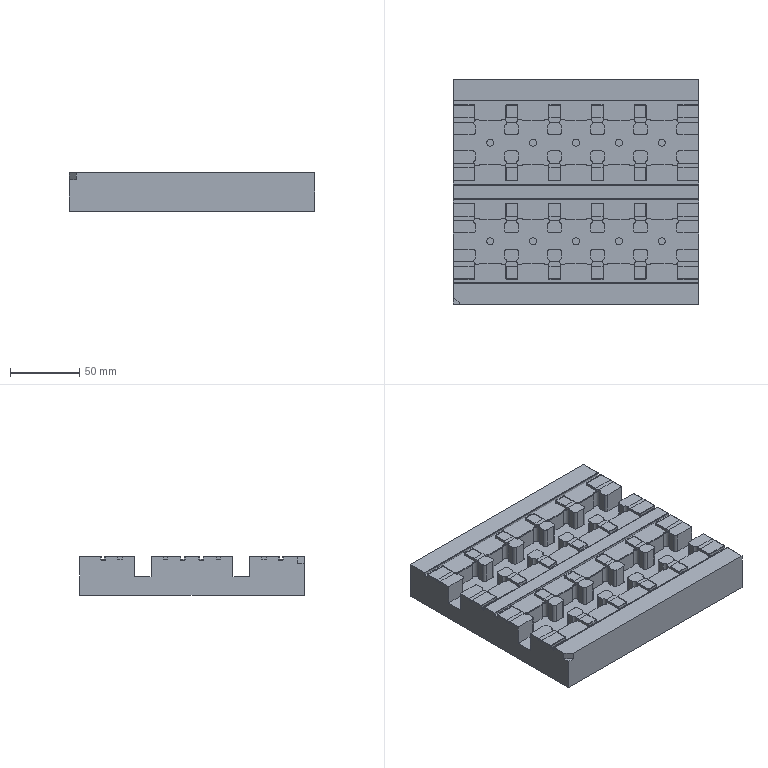NC program | NX | posted by the shop | part box 177 x 162 x 28 mm
Lines 234194 to 237122 of 240480:
N6 T04 M06
(D3  D=3. R=0. H=04 ce=0.05 di=0.02)
(D.N=04 MAX_Z=43. MIN_Z=26.22 Time=39.16M)
T11
G00 G90 G54 X94. Y64.65 M03 S5000
G43 H04 Z43.
M08
Z27.94
G01 X88.5 F1500.
X-88.5
X-94.
G00 Z27.88
G01 X-88.5
X88.5
X94.
G00 Z27.82
G01 X88.5
X-88.5
X-94.
G00 Z27.76
G01 X-88.5
X88.5
X94.
G00 Z27.7
G01 X88.5
X-88.5
X-94.
G00 Z27.64
G01 X-88.5
X88.5
X94.
G00 Z27.58
G01 X88.5
X-88.5
X-94.
G00 Z27.52
G01 X-88.5
X88.5
X94.
G00 Z27.46
G01 X88.5
X-88.5
X-94.
G00 Z27.4
G01 X-88.5
X88.5
X94.
G00 Z27.34
G01 X88.5
X-88.5
X-94.
G00 Z27.28
G01 X-88.5
X88.5
X94.
G00 Z27.22
G01 X88.5
X-88.5
X-94.
G00 Z27.16
G01 X-88.5
X88.5
X94.
G00 Z27.1
G01 X88.5
X-88.5
X-94.
G00 Z27.04
G01 X-88.5
X88.5
X94.
G00 Z26.98
G01 X88.5
X-88.5
X-94.
G00 Z26.92
G01 X-88.5
X88.5
X94.
G00 Z26.86
G01 X88.5
X-88.5
X-94.
G00 Z26.8
G01 X-88.5
X88.5
X94.
G00 Z26.74
G01 X88.5
X-88.5
X-94.
G00 Z26.68
G01 X-88.5
X88.5
X94.
G00 Z26.62
G01 X88.5
X-88.5
X-94.
G00 Z26.56
G01 X-88.5
X88.5
X94.
G00 Z26.5
G01 X88.5
X-88.5
X-94.
G00 Z26.44
G01 X-88.5
X88.5
X94.
G00 Z26.38
G01 X88.5
X-88.5
X-94.
G00 Z26.32
G01 X-88.5
X88.5
X94.
G00 Z26.26
G01 X88.5
X-88.5
X-94.
G00 Z26.22
G01 X-88.5
X88.5
X94.
G00 Z43.
X-94. Y6.55
Z27.94
G01 X-88.5
X88.5
X94.
G00 Z27.88
G01 X88.5
X-88.5
X-94.
G00 Z27.82
G01 X-88.5
X88.5
X94.
G00 Z27.76
G01 X88.5
X-88.5
X-94.
G00 Z27.7
G01 X-88.5
X88.5
X94.
G00 Z27.64
G01 X88.5
X-88.5
X-94.
G00 Z27.58
G01 X-88.5
X88.5
X94.
G00 Z27.52
G01 X88.5
X-88.5
X-94.
G00 Z27.46
G01 X-88.5
X88.5
X94.
G00 Z27.4
G01 X88.5
X-88.5
X-94.
G00 Z27.34
G01 X-88.5
X88.5
X94.
G00 Z27.28
G01 X88.5
X-88.5
X-94.
G00 Z27.22
G01 X-88.5
X88.5
X94.
G00 Z27.16
G01 X88.5
X-88.5
X-94.
G00 Z27.1
G01 X-88.5
X88.5
X94.
G00 Z27.04
G01 X88.5
X-88.5
X-94.
G00 Z26.98
G01 X-88.5
X88.5
X94.
G00 Z26.92
G01 X88.5
X-88.5
X-94.
G00 Z26.86
G01 X-88.5
X88.5
X94.
G00 Z26.8
G01 X88.5
X-88.5
X-94.
G00 Z26.74
G01 X-88.5
X88.5
X94.
G00 Z26.68
G01 X88.5
X-88.5
X-94.
G00 Z26.62
G01 X-88.5
X88.5
X94.
G00 Z26.56
G01 X88.5
X-88.5
X-94.
G00 Z26.5
G01 X-88.5
X88.5
X94.
G00 Z26.44
G01 X88.5
X-88.5
X-94.
G00 Z26.38
G01 X-88.5
X88.5
X94.
G00 Z26.32
G01 X88.5
X-88.5
X-94.
G00 Z26.26
G01 X-88.5
X88.5
X94.
G00 Z26.22
G01 X88.5
X-88.5
X-94.
G00 Z43.
X94. Y-6.55
Z27.94
G01 X88.5
X-88.5
X-94.
G00 Z27.88
G01 X-88.5
X88.5
X94.
G00 Z27.82
G01 X88.5
X-88.5
X-94.
G00 Z27.76
G01 X-88.5
X88.5
X94.
G00 Z27.7
G01 X88.5
X-88.5
X-94.
G00 Z27.64
G01 X-88.5
X88.5
X94.
G00 Z27.58
G01 X88.5
X-88.5
X-94.
G00 Z27.52
G01 X-88.5
X88.5
X94.
G00 Z27.46
G01 X88.5
X-88.5
X-94.
G00 Z27.4
G01 X-88.5
X88.5
X94.
G00 Z27.34
G01 X88.5
X-88.5
X-94.
G00 Z27.28
G01 X-88.5
X88.5
X94.
G00 Z27.22
G01 X88.5
X-88.5
X-94.
G00 Z27.16
G01 X-88.5
X88.5
X94.
G00 Z27.1
G01 X88.5
X-88.5
X-94.
G00 Z27.04
G01 X-88.5
X88.5
X94.
G00 Z26.98
G01 X88.5
X-88.5
X-94.
G00 Z26.92
G01 X-88.5
X88.5
X94.
G00 Z26.86
G01 X88.5
X-88.5
X-94.
G00 Z26.8
G01 X-88.5
X88.5
X94.
G00 Z26.74
G01 X88.5
X-88.5
X-94.
G00 Z26.68
G01 X-88.5
X88.5
X94.
G00 Z26.62
G01 X88.5
X-88.5
X-94.
G00 Z26.56
G01 X-88.5
X88.5
X94.
G00 Z26.5
G01 X88.5
X-88.5
X-94.
G00 Z26.44
G01 X-88.5
X88.5
X94.
G00 Z26.38
G01 X88.5
X-88.5
X-94.
G00 Z26.32
G01 X-88.5
X88.5
X94.
G00 Z26.26
G01 X88.5
X-88.5
X-94.
G00 Z26.22
G01 X-88.5
X88.5
X94.
G00 Z43.
X-94. Y-64.65
Z27.94
G01 X-88.5
X88.5
X94.
G00 Z27.88
G01 X88.5
X-88.5
X-94.
G00 Z27.82
G01 X-88.5
X88.5
X94.
G00 Z27.76
G01 X88.5
X-88.5
X-94.
G00 Z27.7
G01 X-88.5
X88.5
X94.
G00 Z27.64
G01 X88.5
X-88.5
X-94.
G00 Z27.58
G01 X-88.5
X88.5
X94.
G00 Z27.52
G01 X88.5
X-88.5
X-94.
G00 Z27.46
G01 X-88.5
X88.5
X94.
G00 Z27.4
G01 X88.5
X-88.5
X-94.
G00 Z27.34
G01 X-88.5
X88.5
X94.
G00 Z27.28
G01 X88.5
X-88.5
X-94.
G00 Z27.22
G01 X-88.5
X88.5
X94.
G00 Z27.16
G01 X88.5
X-88.5
X-94.
G00 Z27.1
G01 X-88.5
X88.5
X94.
G00 Z27.04
G01 X88.5
X-88.5
X-94.
G00 Z26.98
G01 X-88.5
X88.5
X94.
G00 Z26.92
G01 X88.5
X-88.5
X-94.
G00 Z26.86
G01 X-88.5
X88.5
X94.
G00 Z26.8
G01 X88.5
X-88.5
X-94.
G00 Z26.74
G01 X-88.5
X88.5
X94.
G00 Z26.68
G01 X88.5
X-88.5
X-94.
G00 Z26.62
G01 X-88.5
X88.5
X94.
G00 Z26.56
G01 X88.5
X-88.5
X-94.
G00 Z26.5
G01 X-88.5
X88.5
X94.
G00 Z26.44
G01 X88.5
X-88.5
X-94.
G00 Z26.38
G01 X-88.5
X88.5
X94.
G00 Z26.32
G01 X88.5
X-88.5
X-94.
G00 Z26.26
G01 X-88.5
X88.5
X94.
G00 Z26.22
G01 X88.5
X-88.5
X-94.
G00 Z43.
G00 G90 X94. Y52. M03 S5000
Z43.
Z27.94
G01 X88.5 F1000.
X-88.5
X-94.
G00 Z27.88
G01 X-88.5
X88.5
X94.
G00 Z27.82
G01 X88.5
X-88.5
X-94.
G00 Z27.76
G01 X-88.5
X88.5
X94.
G00 Z27.7
G01 X88.5
X-88.5
X-94.
G00 Z27.64
G01 X-88.5
X88.5
X94.
G00 Z27.58
G01 X88.5
X-88.5
X-94.
G00 Z27.52
G01 X-88.5
X88.5
X94.
G00 Z27.46
G01 X88.5
X-88.5
X-94.
G00 Z27.4
G01 X-88.5
X88.5
X94.
G00 Z27.34
G01 X88.5
X-88.5
X-94.
G00 Z27.28
G01 X-88.5
X88.5
X94.
G00 Z27.22
G01 X88.5
X-88.5
X-94.
G00 Z27.16
G01 X-88.5
X88.5
X94.
G00 Z27.1
G01 X88.5
X-88.5
X-94.
G00 Z27.04
G01 X-88.5
X88.5
X94.
G00 Z26.98
G01 X88.5
X-88.5
X-94.
G00 Z26.92
G01 X-88.5
X88.5
X94.
G00 Z26.86
G01 X88.5
X-88.5
X-94.
G00 Z26.8
G01 X-88.5
X88.5
X94.
G00 Z26.74
G01 X88.5
X-88.5
X-94.
G00 Z26.68
G01 X-88.5
X88.5
X94.
G00 Z26.62
G01 X88.5
X-88.5
X-94.
G00 Z26.56
G01 X-88.5
X88.5
X94.
G00 Z26.5
G01 X88.5
X-88.5
X-94.
G00 Z26.44
G01 X-88.5
X88.5
X94.
G00 Z26.38
G01 X88.5
X-88.5
X-94.
G00 Z26.32
G01 X-88.5
X88.5
X94.
G00 Z26.26
G01 X88.5
X-88.5
X-94.
G00 Z26.22
G01 X-88.5
X88.5
X94.
G00 Z43.
Y19.2
Z27.94
G01 X88.5
X-88.5
X-94.
G00 Z27.88
G01 X-88.5
X88.5
X94.
G00 Z27.82
G01 X88.5
X-88.5
X-94.
G00 Z27.76
G01 X-88.5
X88.5
X94.
G00 Z27.7
G01 X88.5
X-88.5
X-94.
G00 Z27.64
G01 X-88.5
X88.5
X94.
G00 Z27.58
G01 X88.5
X-88.5
X-94.
G00 Z27.52
G01 X-88.5
X88.5
X94.
G00 Z27.46
G01 X88.5
X-88.5
X-94.
G00 Z27.4
G01 X-88.5
X88.5
X94.
G00 Z27.34
G01 X88.5
X-88.5
X-94.
G00 Z27.28
G01 X-88.5
X88.5
X94.
G00 Z27.22
G01 X88.5
X-88.5
X-94.
G00 Z27.16
G01 X-88.5
X88.5
X94.
G00 Z27.1
G01 X88.5
X-88.5
X-94.
G00 Z27.04
G01 X-88.5
X88.5
X94.
G00 Z26.98
G01 X88.5
X-88.5
X-94.
G00 Z26.92
G01 X-88.5
X88.5
X94.
G00 Z26.86
G01 X88.5
X-88.5
X-94.
G00 Z26.8
G01 X-88.5
X88.5
X94.
G00 Z26.74
G01 X88.5
X-88.5
X-94.
G00 Z26.68
G01 X-88.5
X88.5
X94.
G00 Z26.62
G01 X88.5
X-88.5
X-94.
G00 Z26.56
G01 X-88.5
X88.5
X94.
G00 Z26.5
G01 X88.5
X-88.5
X-94.
G00 Z26.44
G01 X-88.5
X88.5
X94.
G00 Z26.38
G01 X88.5
X-88.5
X-94.
G00 Z26.32
G01 X-88.5
X88.5
X94.
G00 Z26.26
G01 X88.5
X-88.5
X-94.
G00 Z26.22
G01 X-88.5
X88.5
X94.
G00 Z43.
Y-19.2
Z27.94
G01 X88.5
X-88.5
X-94.
G00 Z27.88
G01 X-88.5
X88.5
X94.
G00 Z27.82
G01 X88.5
X-88.5
X-94.
G00 Z27.76
G01 X-88.5
X88.5
X94.
G00 Z27.7
G01 X88.5
X-88.5
X-94.
G00 Z27.64
G01 X-88.5
X88.5
X94.
G00 Z27.58
G01 X88.5
X-88.5
X-94.
G00 Z27.52
G01 X-88.5
X88.5
X94.
G00 Z27.46
G01 X88.5
X-88.5
X-94.
G00 Z27.4
G01 X-88.5
X88.5
X94.
G00 Z27.34
G01 X88.5
X-88.5
X-94.
G00 Z27.28
G01 X-88.5
X88.5
X94.
G00 Z27.22
G01 X88.5
X-88.5
X-94.
G00 Z27.16
G01 X-88.5
X88.5
X94.
G00 Z27.1
G01 X88.5
X-88.5
X-94.
G00 Z27.04
G01 X-88.5
X88.5
X94.
G00 Z26.98
G01 X88.5
X-88.5
X-94.
G00 Z26.92
G01 X-88.5
X88.5
X94.
G00 Z26.86
G01 X88.5
X-88.5
X-94.
G00 Z26.8
G01 X-88.5
X88.5
X94.
G00 Z26.74
G01 X88.5
X-88.5
X-94.
G00 Z26.68
G01 X-88.5
X88.5
X94.
G00 Z26.62
G01 X88.5
X-88.5
X-94.
G00 Z26.56
G01 X-88.5
X88.5
X94.
G00 Z26.5
G01 X88.5
X-88.5
X-94.
G00 Z26.44
G01 X-88.5
X88.5
X94.
G00 Z26.38
G01 X88.5
X-88.5
X-94.
G00 Z26.32
G01 X-88.5
X88.5
X94.
G00 Z26.26
G01 X88.5
X-88.5
X-94.
G00 Z26.22
G01 X-88.5
X88.5
X94.
G00 Z43.
Y-52.
Z27.94
G01 X88.5
X-88.5
X-94.
G00 Z27.88
G01 X-88.5
X88.5
X94.
G00 Z27.82
G01 X88.5
X-88.5
X-94.
G00 Z27.76
G01 X-88.5
X88.5
X94.
G00 Z27.7
G01 X88.5
X-88.5
X-94.
G00 Z27.64
G01 X-88.5
X88.5
X94.
G00 Z27.58
G01 X88.5
X-88.5
X-94.
G00 Z27.52
G01 X-88.5
X88.5
X94.
G00 Z27.46
G01 X88.5
X-88.5
X-94.
G00 Z27.4
G01 X-88.5
X88.5
X94.
G00 Z27.34
G01 X88.5
X-88.5
X-94.
G00 Z27.28
G01 X-88.5
X88.5
X94.
G00 Z27.22
G01 X88.5
X-88.5
X-94.
G00 Z27.16
G01 X-88.5
X88.5
X94.
G00 Z27.1
G01 X88.5
X-88.5
X-94.
G00 Z27.04
G01 X-88.5
X88.5
X94.
G00 Z26.98
G01 X88.5
X-88.5
X-94.
G00 Z26.92
G01 X-88.5
X88.5
X94.
G00 Z26.86
G01 X88.5
X-88.5
X-94.
G00 Z26.8
G01 X-88.5
X88.5
X94.
G00 Z26.74
G01 X88.5
X-88.5
X-94.
G00 Z26.68
G01 X-88.5
X88.5
X94.
G00 Z26.62
G01 X88.5
X-88.5
X-94.
G00 Z26.56
G01 X-88.5
X88.5
X94.
G00 Z26.5
G01 X88.5
X-88.5
X-94.
G00 Z26.44
G01 X-88.5
X88.5
X94.
G00 Z26.38
G01 X88.5
X-88.5
X-94.
G00 Z26.32
G01 X-88.5
X88.5
X94.
G00 Z26.26
G01 X88.5
X-88.5
X-94.
G00 Z26.22
G01 X-88.5
X88.5
X94.
G00 Z43.
G00 G90 X71.15 Y64.05 M03 S5000
Z40.
Z27.25
G01 Z26.25 F1000.
G41 D04
X71.35
G03 X71.95 Y64.65 I0.0 J.6
G01 X52.05
Y52.05
X71.95
Y64.65
X71.55
G03 X70.95 Y64.05 I0.0 J-.6
G01 G40 Y63.85
Z27.25
G00 Z40.
X40.15 Y64.05
Z27.25
G01 Z26.25
G41 D04
X40.35
G03 X40.95 Y64.65 I0.0 J.6
G01 X21.05
Y52.05
X40.95
Y64.65
X40.55
G03 X39.95 Y64.05 I0.0 J-.6
G01 G40 Y63.85
Z27.25
G00 Z40.
X9.15 Y64.05
Z27.25
G01 Z26.25
G41 D04
X9.35
G03 X9.95 Y64.65 I0.0 J.6
G01 X-9.95
Y52.05
X9.95
Y64.65
X9.55
G03 X8.95 Y64.05 I0.0 J-.6
G01 G40 Y63.85
Z27.25
G00 Z40.
X-21.85 Y64.05
Z27.25
G01 Z26.25
G41 D04
X-21.65
G03 X-21.05 Y64.65 I0.0 J.6
G01 X-40.95
Y52.05
X-21.05
Y64.65
X-21.45
G03 X-22.05 Y64.05 I0.0 J-.6
G01 G40 Y63.85
Z27.25
G00 Z40.
X-52.85 Y64.05
Z27.25
G01 Z26.25
G41 D04
X-52.65
G03 X-52.05 Y64.65 I0.0 J.6
G01 X-71.95
Y52.05
X-52.05
Y64.65
X-52.45
G03 X-53.05 Y64.05 I0.0 J-.6
G01 G40 Y63.85
Z27.25
G00 Z40.
X-52.85 Y18.55
Z27.25
G01 Z26.25
G41 D04
X-52.65
G03 X-52.05 Y19.15 I0.0 J.6
G01 X-71.95
Y6.55
X-52.05
Y19.15
X-52.45
G03 X-52.73 Y19.081 I0.0 J-.6
G01 G40 X-52.907 Y18.987
Z27.25
G00 Z40.
X-21.85 Y18.55
Z27.25
G01 Z26.25
G41 D04
X-21.65
G03 X-21.05 Y19.15 I0.0 J.6
G01 X-40.95
Y6.55
X-21.05
Y19.15
X-21.45
G03 X-21.73 Y19.081 I0.0 J-.6
G01 G40 X-21.907 Y18.987
Z27.25
G00 Z40.
X9.15 Y18.55
Z27.25
G01 Z26.25
G41 D04
X9.35
G03 X9.95 Y19.15 I0.0 J.6
G01 X-9.95
Y6.55
X9.95
Y19.15
X9.55
G03 X9.27 Y19.081 I0.0 J-.6
G01 G40 X9.093 Y18.987
Z27.25
G00 Z40.
X40.15 Y18.55
Z27.25
G01 Z26.25
G41 D04
X40.35
G03 X40.95 Y19.15 I0.0 J.6
G01 X21.05
Y6.55
X40.95
Y19.15
X40.55
G03 X40.27 Y19.081 I0.0 J-.6
G01 G40 X40.093 Y18.987
Z27.25
G00 Z40.
X71.15 Y18.55
Z27.25
G01 Z26.25
G41 D04
X71.35
G03 X71.95 Y19.15 I0.0 J.6
G01 X52.05
Y6.55
X71.95
Y19.15
X71.55
G03 X71.27 Y19.081 I0.0 J-.6
G01 G40 X71.093 Y18.987
Z27.25
G00 Z40.
X-52.85 Y-7.15
Z27.25
G01 Z26.25
G41 D04
X-52.65
G03 X-52.05 Y-6.55 I0.0 J.6
G01 X-71.95
Y-19.15
X-52.05
Y-6.55
X-52.45
G03 X-53.05 Y-7.15 I0.0 J-.6
G01 G40 Y-7.35
Z27.25
G00 Z40.
X-21.85 Y-7.15
Z27.25
G01 Z26.25
G41 D04
X-21.65
G03 X-21.05 Y-6.55 I0.0 J.6
G01 X-40.95
Y-19.15
X-21.05
Y-6.55
X-21.45
G03 X-22.05 Y-7.15 I0.0 J-.6
G01 G40 Y-7.35
Z27.25
G00 Z40.
X-8.976 Y-18.55
Z27.25
G01 Z26.25
G41 D04
X-9.35
G03 X-9.95 Y-19.15 I0.0 J-.6
G01 X9.95
Y-6.55
X-9.95
Y-19.15
X-9.55
G03 X-9.27 Y-19.081 I0.0 J.6
G01 G40 X-9.093 Y-18.987
Z27.25
G00 Z40.
X22.024 Y-18.55
Z27.25
G01 Z26.25
G41 D04
X21.65
G03 X21.05 Y-19.15 I0.0 J-.6
G01 X40.95
Y-6.55
X21.05
Y-19.15
X21.45
G03 X21.73 Y-19.081 I0.0 J.6
G01 G40 X21.907 Y-18.987
Z27.25
G00 Z40.
X52.85 Y-18.55
Z27.25
G01 Z26.25
G41 D04
X52.65
G03 X52.05 Y-19.15 I0.0 J-.6
G01 X71.95
Y-6.55
X52.05
Y-19.15
X52.45
G03 X52.73 Y-19.081 I0.0 J.6
G01 G40 X52.907 Y-18.987
Z27.25
G00 Z40.
X52.65 Y-63.85
Z27.25
G01 Z26.25
G41 D04
Y-64.05
G03 X52.05 Y-64.65 I0.0 J-.6
G01 X71.95
Y-52.05
X52.05
Y-64.65
X52.45
G03 X53.05 Y-64.05 I0.0 J.6
G01 G40 Y-63.85
Z27.25
G00 Z40.
X21.65
Z27.25
G01 Z26.25
G41 D04
Y-64.05
G03 X21.05 Y-64.65 I0.0 J-.6
G01 X40.95
Y-52.05
X21.05
Y-64.65
X21.45
G03 X22.05 Y-64.05 I0.0 J.6
G01 G40 Y-63.85
Z27.25
G00 Z40.
X-9.15 Y-64.05
Z27.25
G01 Z26.25
G41 D04
X-9.35
G03 X-9.95 Y-64.65 I0.0 J-.6
G01 X9.95
Y-52.05
X-9.95
Y-64.65
X-9.55
G03 X-8.95 Y-64.05 I0.0 J.6
G01 G40 Y-63.85
Z27.25
G00 Z40.
X-40.15 Y-64.05
Z27.25
G01 Z26.25
G41 D04
X-40.35
G03 X-40.95 Y-64.65 I0.0 J-.6
G01 X-21.05
Y-52.05
X-40.95
Y-64.65
X-40.55
G03 X-39.95 Y-64.05 I0.0 J.6
G01 G40 Y-63.85
Z27.25
G00 Z40.
X-71.194 Y-63.924
Z27.25
G01 Z26.25
G41 D04
X-71.35 Y-64.05
G03 X-71.95 Y-64.65 I0.0 J-.6
G01 X-52.05
Y-52.05
X-71.95
Y-64.65
X-71.55
G03 X-70.95 Y-64.05 I0.0 J.6
G01 G40 Y-63.85
Z27.25
G00 Z40.
G91 G28 Z0.0
M05
M09
G91 G28 Z0.0
M01
N7 T11 M06
(D10-J  D=10. R=0. H=11 ce=0.00 di=0.00)
(MAX_Z=43. MIN_Z=28. Time=6.55M)
T17
G00 G90 G54 X-98.5 Y81.086 M03 S3000
G43 H11 Z43.
M08
Z30.
G01 Z28. F1000.
X-93.5
X93.5
Y76.171
X-93.5
Y71.257
X93.5
Y66.343
X-93.5
Y61.429
X93.5
Y56.514
X-93.5
Y51.6
X93.5
Y46.686
X-93.5
Y41.771
X93.5
Y36.857
X-93.5
Y31.943
X93.5
Y27.029
X-93.5
Y22.114
X93.5
Y17.2
X-93.5
Y12.286
X93.5
Y7.371
X-93.5
Y2.457
X93.5
Y-2.457
X-93.5
Y-7.371
X93.5
Y-12.286
X-93.5
Y-17.2
X93.5
Y-22.114
X-93.5
Y-27.029
X93.5
Y-31.943
X-93.5
Y-36.857
X93.5
Y-41.771
X-93.5
Y-46.686
X93.5
Y-51.6
X-93.5
Y-56.514
X93.5
Y-61.429
X-93.5
Y-66.343
X93.5
Y-71.257
X-93.5
Y-76.171
X93.5
Y-81.086
X-93.5
X-98.5
Z30.
G00 Z43.
G91 G28 Z0.0
M05
M09
G91 G28 Z0.0
M01
N8 T17 M06
(C6SpotDrill  D=6. R=0. H=17 ce=0.00 di=0.00)
(MAX_Z=43. MIN_Z=12.45 Time=0.40M)
T03
G00 G90 G54 X62. Y-35.6 M03 S1500
G43 H17 Z43.
M08
G98 G81 X62. Y-35.6 Z12.45 R14.25 F50.
X31.
X0.0
X-31.
X-62.
G80
G00 Z43.
G00 G90 X-62. Y35.6 M03 S1500
Z43.
G98 G81 X-62. Y35.6 Z12.45 R14.25 F50.
X-31.
X0.0
X31.
X62.
G80
G00 Z43.
G91 G28 Z0.0
M05
M09
G91 G28 Z0.0
M01
N9 T03 M06
(ZT5.1 D=5.1 DR_a=118 H=03)
(MAX_Z=43. MIN_Z=1.35 Time=2.59M)
T14
G00 G90 G54 X-62. Y-35.6 M03 S1000
G43 H03 Z43.
M08
G98 G83 X-62. Y-35.6 Z1.6 R14.25 F50. Q1.
X-31.
X0.0
X31.
X62.
G98 G83 X62. Y35.6 Z1.35 R14.25 Q1.
X31.
X0.0
X-31.
X-62.
G80
G00 Z43.
G91 G28 Z0.0
M05
M09
G91 G28 Z0.0
M01
N10 T14 M06
(D4-J  D=4. R=0. H=14 ce=0.30 di=0.00)
(MAX_Z=43. MIN_Z=13.5 Time=3.20M)
T13
G00 G90 G54 X-93.5 Y35.6 M03 S4000
G43 H14 Z43.
M08
Z14.
G01 Z13.5 F900.
X-88.9
Y39.3 F1000.
X-74.25
G03 X-69.95 Y43.6 I0.0 J4.3
G01 Y47.931
G03 X-70.334 Y49.204 I-2.3 J0.0
X-69.561 Y49.07 I.773 J2.166
G01 X-54.439
G03 X-53.666 Y49.204 I0.0 J2.3
X-54.05 Y47.931 I1.916 J-1.273
G01 Y43.6
G03 X-49.75 Y39.3 I4.3 J0.0
G01 X-43.25
G03 X-38.95 Y43.6 I0.0 J4.3
G01 Y47.931
G03 X-39.334 Y49.204 I-2.3 J0.0
X-38.561 Y49.07 I.773 J2.166
G01 X-23.439
G03 X-22.666 Y49.204 I0.0 J2.3
X-23.05 Y47.931 I1.916 J-1.273
G01 Y43.6
G03 X-18.75 Y39.3 I4.3 J0.0
G01 X-12.25
G03 X-7.95 Y43.6 I0.0 J4.3
G01 Y47.931
G03 X-8.334 Y49.204 I-2.3 J0.0
X-7.561 Y49.07 I.773 J2.166
G01 X7.561
G03 X8.334 Y49.204 I0.0 J2.3
X7.95 Y47.931 I1.916 J-1.273
G01 Y43.6
G03 X12.25 Y39.3 I4.3 J0.0
G01 X18.75
G03 X23.05 Y43.6 I0.0 J4.3
G01 Y47.931
G03 X22.666 Y49.204 I-2.3 J0.0
X23.439 Y49.07 I.773 J2.166
G01 X38.561
G03 X39.334 Y49.204 I0.0 J2.3
X38.95 Y47.931 I1.916 J-1.273
G01 Y43.6
G03 X43.25 Y39.3 I4.3 J0.0
G01 X49.75
G03 X54.05 Y43.6 I0.0 J4.3
G01 Y47.931
G03 X53.666 Y49.204 I-2.3 J0.0
X54.439 Y49.07 I.773 J2.166
G01 X69.561
G03 X70.334 Y49.204 I0.0 J2.3
X69.95 Y47.931 I1.916 J-1.273
G01 Y43.6
G03 X74.25 Y39.3 I4.3 J0.0
G01 X88.9
Y31.9
X74.25
G03 X69.95 Y27.6 I0.0 J-4.3
G01 Y23.269
G03 X70.334 Y21.996 I2.3 J0.0
X69.561 Y22.13 I-.773 J-2.166
G01 X54.439
G03 X53.666 Y21.996 I0.0 J-2.3
X54.05 Y23.269 I-1.916 J1.273
G01 Y27.6
G03 X49.75 Y31.9 I-4.3 J0.0
G01 X43.25
G03 X38.95 Y27.6 I0.0 J-4.3
G01 Y23.269
G03 X39.334 Y21.996 I2.3 J0.0
X38.561 Y22.13 I-.773 J-2.166
G01 X23.439
G03 X22.666 Y21.996 I0.0 J-2.3
X23.05 Y23.269 I-1.916 J1.273
G01 Y27.6
G03 X18.75 Y31.9 I-4.3 J0.0
G01 X12.25
G03 X7.95 Y27.6 I0.0 J-4.3
G01 Y23.269
G03 X8.334 Y21.996 I2.3 J0.0
X7.561 Y22.13 I-.773 J-2.166
G01 X-7.561
G03 X-8.334 Y21.996 I0.0 J-2.3
X-7.95 Y23.269 I-1.916 J1.273
G01 Y27.6
G03 X-12.25 Y31.9 I-4.3 J0.0
G01 X-18.75
G03 X-23.05 Y27.6 I0.0 J-4.3
G01 Y23.269
G03 X-22.666 Y21.996 I2.3 J0.0
X-23.439 Y22.13 I-.773 J-2.166
G01 X-38.561
G03 X-39.334 Y21.996 I0.0 J-2.3
X-38.95 Y23.269 I-1.916 J1.273
G01 Y27.6
G03 X-43.25 Y31.9 I-4.3 J0.0
G01 X-49.75
G03 X-54.05 Y27.6 I0.0 J-4.3
G01 Y23.269
G03 X-53.666 Y21.996 I2.3 J0.0
X-54.439 Y22.13 I-.773 J-2.166
G01 X-69.561
G03 X-70.334 Y21.996 I0.0 J-2.3
X-69.95 Y23.269 I-1.916 J1.273
G01 Y27.6
G03 X-74.25 Y31.9 I-4.3 J0.0
G01 X-88.9
Y35.6
X-86.8
Y37.2
X-74.25
G03 X-67.85 Y43.6 I0.0 J6.4
G01 Y46.97
X-56.15
Y43.6
G03 X-49.75 Y37.2 I6.4 J0.0
G01 X-43.25
G03 X-36.85 Y43.6 I0.0 J6.4
G01 Y46.97
X-25.15
Y43.6
G03 X-18.75 Y37.2 I6.4 J0.0
G01 X-12.25
G03 X-5.85 Y43.6 I0.0 J6.4
G01 Y46.97
X5.85
Y43.6
G03 X12.25 Y37.2 I6.4 J0.0
G01 X18.75
G03 X25.15 Y43.6 I0.0 J6.4
G01 Y46.97
X36.85
Y43.6
G03 X43.25 Y37.2 I6.4 J0.0
G01 X49.75
G03 X56.15 Y43.6 I0.0 J6.4
G01 Y46.97
X67.85
Y43.6
G03 X74.25 Y37.2 I6.4 J0.0
G01 X86.8
Y34.
X74.25
G03 X67.85 Y27.6 I0.0 J-6.4
G01 Y24.23
X56.15
Y27.6
G03 X52.91 Y33.165 I-6.4 J0.0
G01 X54.293 Y35.6
G03 X58.95 Y43.6 I-4.543 J8.
G01 Y44.17
X65.05
Y43.6
G03 X69.707 Y35.6 I9.2 J0.0
X65.05 Y27.6 I4.543 J-8.
G01 Y27.03
X58.95
Y27.6
G03 X54.293 Y35.6 I-9.2 J0.0
G01 X58.694
G03 X61.541 Y41.37 I-8.944 J8.
G01 X62.459
G03 X65.306 Y35.6 I11.791 J2.23
X62.459 Y29.83 I8.944 J-8.
G01 X61.541
G03 X58.694 Y35.6 I-11.791 J-2.23
G01 X60.995
G03 X62. Y37.246 I-11.245 J8.
X63.005 Y35.6 I12.25 J6.354
X62. Y33.954 I11.245 J-8.
X60.995 Y35.6 I-12.25 J-6.354
G01 X54.293
X52.91 Y33.165
G03 X49.75 Y34. I-3.16 J-5.565
G01 X43.25
G03 X36.85 Y27.6 I0.0 J-6.4
G01 Y24.23
X25.15
Y27.6
G03 X21.91 Y33.165 I-6.4 J0.0
G01 X23.293 Y35.6
G03 X27.95 Y43.6 I-4.543 J8.
G01 Y44.17
X34.05
Y43.6
G03 X38.707 Y35.6 I9.2 J0.0
X34.05 Y27.6 I4.543 J-8.
G01 Y27.03
X27.95
Y27.6
G03 X23.293 Y35.6 I-9.2 J0.0
G01 X27.694
G03 X30.541 Y41.37 I-8.944 J8.
G01 X31.459
G03 X34.306 Y35.6 I11.791 J2.23
X31.459 Y29.83 I8.944 J-8.
G01 X30.541
G03 X27.694 Y35.6 I-11.791 J-2.23
G01 X29.995
G03 X31. Y37.246 I-11.245 J8.
X32.005 Y35.6 I12.25 J6.354
X31. Y33.954 I11.245 J-8.
X29.995 Y35.6 I-12.25 J-6.354
G01 X23.293
X21.91 Y33.165
G03 X18.75 Y34. I-3.16 J-5.565
G01 X12.25
G03 X5.85 Y27.6 I0.0 J-6.4
G01 Y24.23
X-5.85
Y27.6
G03 X-9.09 Y33.165 I-6.4 J0.0
G01 X-7.707 Y35.6
G03 X-3.05 Y43.6 I-4.543 J8.
G01 Y44.17
X3.05
Y43.6
G03 X7.707 Y35.6 I9.2 J0.0
X3.05 Y27.6 I4.543 J-8.
G01 Y27.03
X-3.05
Y27.6
G03 X-7.707 Y35.6 I-9.2 J0.0
G01 X-3.306
G03 X-.459 Y41.37 I-8.944 J8.
G01 X.459
G03 X3.306 Y35.6 I11.791 J2.23
X.459 Y29.83 I8.944 J-8.
G01 X-.459
G03 X-3.306 Y35.6 I-11.791 J-2.23
G01 X-1.005
G03 X0.0 Y37.246 I-11.245 J8.
X1.005 Y35.6 I12.25 J6.354
X0.0 Y33.954 I11.245 J-8.
X-1.005 Y35.6 I-12.25 J-6.354
G01 X-7.707
X-9.09 Y33.165
G03 X-12.25 Y34. I-3.16 J-5.565
G01 X-18.75
G03 X-25.15 Y27.6 I0.0 J-6.4
G01 Y24.23
X-36.85
Y27.6
G03 X-40.09 Y33.165 I-6.4 J0.0
G01 X-38.707 Y35.6
G03 X-34.05 Y43.6 I-4.543 J8.
G01 Y44.17
X-27.95
Y43.6
G03 X-23.293 Y35.6 I9.2 J0.0
X-27.95 Y27.6 I4.543 J-8.
G01 Y27.03
X-34.05
Y27.6
G03 X-38.707 Y35.6 I-9.2 J0.0
G01 X-34.306
G03 X-31.459 Y41.37 I-8.944 J8.
G01 X-30.541
G03 X-27.694 Y35.6 I11.791 J2.23
X-30.541 Y29.83 I8.944 J-8.
G01 X-31.459
G03 X-34.306 Y35.6 I-11.791 J-2.23
G01 X-32.005
G03 X-31. Y37.246 I-11.245 J8.
X-29.995 Y35.6 I12.25 J6.354
X-31. Y33.954 I11.245 J-8.
X-32.005 Y35.6 I-12.25 J-6.354
G01 X-38.707
X-40.09 Y33.165
G03 X-43.25 Y34. I-3.16 J-5.565
G01 X-49.75
G03 X-56.15 Y27.6 I0.0 J-6.4
G01 Y24.23
X-67.85
Y27.6
G03 X-71.09 Y33.165 I-6.4 J0.0
G01 X-69.707 Y35.6
G03 X-65.05 Y43.6 I-4.543 J8.
G01 Y44.17
X-58.95
Y43.6
G03 X-54.293 Y35.6 I9.2 J0.0
X-58.95 Y27.6 I4.543 J-8.
G01 Y27.03
X-65.05
Y27.6
G03 X-69.707 Y35.6 I-9.2 J0.0
G01 X-65.306
G03 X-62.459 Y41.37 I-8.944 J8.
G01 X-61.541
G03 X-58.694 Y35.6 I11.791 J2.23
X-61.541 Y29.83 I8.944 J-8.
G01 X-62.459
G03 X-65.306 Y35.6 I-11.791 J-2.23
G01 X-63.005
G03 X-62. Y37.246 I-11.245 J8.
X-60.995 Y35.6 I12.25 J6.354
X-62. Y33.954 I11.245 J-8.
X-63.005 Y35.6 I-12.25 J-6.354
G01 X-69.707
X-71.09 Y33.165
G03 X-74.25 Y34. I-3.16 J-5.565
G01 X-86.8
Y35.6
Y36.1
X-93.5
Z14.
G00 Z43.
G00 G90 X93.5 Y-35.6 M03 S4000
Z43.
Z14.
G01 Z13.5 F900.
X88.9
Y-39.3 F1000.
X74.25
G03 X69.95 Y-43.6 I0.0 J-4.3
G01 Y-47.931
G03 X70.334 Y-49.204 I2.3 J0.0
X69.561 Y-49.07 I-.773 J-2.166
G01 X54.439
G03 X53.666 Y-49.204 I0.0 J-2.3
X54.05 Y-47.931 I-1.916 J1.273
G01 Y-43.6
G03 X49.75 Y-39.3 I-4.3 J0.0
G01 X43.25
G03 X38.95 Y-43.6 I0.0 J-4.3
G01 Y-47.931
G03 X39.334 Y-49.204 I2.3 J0.0
X38.561 Y-49.07 I-.773 J-2.166
G01 X23.439
G03 X22.666 Y-49.204 I0.0 J-2.3
X23.05 Y-47.931 I-1.916 J1.273
G01 Y-43.6
G03 X18.75 Y-39.3 I-4.3 J0.0
G01 X12.25
G03 X7.95 Y-43.6 I0.0 J-4.3
G01 Y-47.931
G03 X8.334 Y-49.204 I2.3 J0.0
X7.561 Y-49.07 I-.773 J-2.166
G01 X-7.561
G03 X-8.334 Y-49.204 I0.0 J-2.3
X-7.95 Y-47.931 I-1.916 J1.273
G01 Y-43.6
G03 X-12.25 Y-39.3 I-4.3 J0.0
G01 X-18.75
G03 X-23.05 Y-43.6 I0.0 J-4.3
G01 Y-47.931
G03 X-22.666 Y-49.204 I2.3 J0.0
X-23.439 Y-49.07 I-.773 J-2.166
G01 X-38.561
G03 X-39.334 Y-49.204 I0.0 J-2.3
X-38.95 Y-47.931 I-1.916 J1.273
G01 Y-43.6
G03 X-43.25 Y-39.3 I-4.3 J0.0
G01 X-49.75
G03 X-54.05 Y-43.6 I0.0 J-4.3
G01 Y-47.931
G03 X-53.666 Y-49.204 I2.3 J0.0
X-54.439 Y-49.07 I-.773 J-2.166
G01 X-69.561
G03 X-70.334 Y-49.204 I0.0 J-2.3
X-69.95 Y-47.931 I-1.916 J1.273
G01 Y-43.6
G03 X-74.25 Y-39.3 I-4.3 J0.0
G01 X-88.9
Y-31.9
X-74.25
G03 X-69.95 Y-27.6 I0.0 J4.3
G01 Y-23.269
G03 X-70.334 Y-21.996 I-2.3 J0.0
X-69.561 Y-22.13 I.773 J2.166
G01 X-54.439
G03 X-53.666 Y-21.996 I0.0 J2.3
X-54.05 Y-23.269 I1.916 J-1.273
G01 Y-27.6
G03 X-49.75 Y-31.9 I4.3 J0.0
G01 X-43.25
G03 X-38.95 Y-27.6 I0.0 J4.3
G01 Y-23.269
G03 X-39.334 Y-21.996 I-2.3 J0.0
X-38.561 Y-22.13 I.773 J2.166
G01 X-23.439
G03 X-22.666 Y-21.996 I0.0 J2.3
X-23.05 Y-23.269 I1.916 J-1.273
G01 Y-27.6
G03 X-18.75 Y-31.9 I4.3 J0.0
G01 X-12.25
G03 X-7.95 Y-27.6 I0.0 J4.3
G01 Y-23.269
G03 X-8.334 Y-21.996 I-2.3 J0.0
X-7.561 Y-22.13 I.773 J2.166
G01 X7.561
G03 X8.334 Y-21.996 I0.0 J2.3
X7.95 Y-23.269 I1.916 J-1.273
G01 Y-27.6
G03 X12.25 Y-31.9 I4.3 J0.0
G01 X18.75
G03 X23.05 Y-27.6 I0.0 J4.3
G01 Y-23.269
G03 X22.666 Y-21.996 I-2.3 J0.0
X23.439 Y-22.13 I.773 J2.166
G01 X38.561
G03 X39.334 Y-21.996 I0.0 J2.3
X38.95 Y-23.269 I1.916 J-1.273
G01 Y-27.6
G03 X43.25 Y-31.9 I4.3 J0.0
G01 X49.75
G03 X54.05 Y-27.6 I0.0 J4.3
G01 Y-23.269
G03 X53.666 Y-21.996 I-2.3 J0.0
X54.439 Y-22.13 I.773 J2.166
G01 X69.561
G03 X70.334 Y-21.996 I0.0 J2.3
X69.95 Y-23.269 I1.916 J-1.273
G01 Y-27.6
G03 X74.25 Y-31.9 I4.3 J0.0
G01 X88.9
Y-35.6
X86.8
Y-37.2
X74.25
G03 X67.85 Y-43.6 I0.0 J-6.4
G01 Y-46.97
X56.15
Y-43.6
G03 X49.75 Y-37.2 I-6.4 J0.0
G01 X43.25
G03 X36.85 Y-43.6 I0.0 J-6.4
G01 Y-46.97
X25.15
Y-43.6
G03 X18.75 Y-37.2 I-6.4 J0.0
G01 X12.25
G03 X5.85 Y-43.6 I0.0 J-6.4
G01 Y-46.97
X-5.85
Y-43.6
G03 X-12.25 Y-37.2 I-6.4 J0.0
G01 X-18.75
G03 X-25.15 Y-43.6 I0.0 J-6.4
G01 Y-46.97
X-36.85
Y-43.6
G03 X-43.25 Y-37.2 I-6.4 J0.0
G01 X-49.75
G03 X-56.15 Y-43.6 I0.0 J-6.4
G01 Y-46.97
X-67.85
Y-43.6
G03 X-74.25 Y-37.2 I-6.4 J0.0
G01 X-86.8
Y-34.
X-74.25
G03 X-67.85 Y-27.6 I0.0 J6.4
G01 Y-24.23
X-56.15
Y-27.6
G03 X-52.91 Y-33.165 I6.4 J0.0
G01 X-54.293 Y-35.6
G03 X-58.95 Y-43.6 I4.543 J-8.
G01 Y-44.17
X-65.05
Y-43.6
G03 X-69.707 Y-35.6 I-9.2 J0.0
X-65.05 Y-27.6 I-4.543 J8.
G01 Y-27.03
X-58.95
Y-27.6
G03 X-54.293 Y-35.6 I9.2 J0.0
G01 X-58.694
G03 X-61.541 Y-41.37 I8.944 J-8.
G01 X-62.459
G03 X-65.306 Y-35.6 I-11.791 J-2.23
X-62.459 Y-29.83 I-8.944 J8.
G01 X-61.541
G03 X-58.694 Y-35.6 I11.791 J2.23
G01 X-60.995
G03 X-62. Y-37.246 I11.245 J-8.
X-63.005 Y-35.6 I-12.25 J-6.354
X-62. Y-33.954 I-11.245 J8.
X-60.995 Y-35.6 I12.25 J6.354
G01 X-54.293
X-52.91 Y-33.165
G03 X-49.75 Y-34. I3.16 J5.565
G01 X-43.25
G03 X-36.85 Y-27.6 I0.0 J6.4
G01 Y-24.23
X-25.15
Y-27.6
G03 X-21.91 Y-33.165 I6.4 J0.0
G01 X-23.293 Y-35.6
G03 X-27.95 Y-43.6 I4.543 J-8.
G01 Y-44.17
X-34.05
Y-43.6
G03 X-38.707 Y-35.6 I-9.2 J0.0
X-34.05 Y-27.6 I-4.543 J8.
G01 Y-27.03
X-27.95
Y-27.6
G03 X-23.293 Y-35.6 I9.2 J0.0
G01 X-27.694
G03 X-30.541 Y-41.37 I8.944 J-8.
G01 X-31.459
G03 X-34.306 Y-35.6 I-11.791 J-2.23
X-31.459 Y-29.83 I-8.944 J8.
G01 X-30.541
G03 X-27.694 Y-35.6 I11.791 J2.23
G01 X-29.995
G03 X-31. Y-37.246 I11.245 J-8.
X-32.005 Y-35.6 I-12.25 J-6.354
X-31. Y-33.954 I-11.245 J8.
X-29.995 Y-35.6 I12.25 J6.354
G01 X-23.293
X-21.91 Y-33.165
G03 X-18.75 Y-34. I3.16 J5.565
G01 X-12.25
G03 X-5.85 Y-27.6 I0.0 J6.4
G01 Y-24.23
X5.85
Y-27.6
G03 X9.09 Y-33.165 I6.4 J0.0
G01 X7.707 Y-35.6
G03 X3.05 Y-43.6 I4.543 J-8.
G01 Y-44.17
X-3.05
Y-43.6
G03 X-7.707 Y-35.6 I-9.2 J0.0
X-3.05 Y-27.6 I-4.543 J8.
G01 Y-27.03
X3.05
Y-27.6
G03 X7.707 Y-35.6 I9.2 J0.0
G01 X3.306
G03 X.459 Y-41.37 I8.944 J-8.
G01 X-.459
G03 X-3.306 Y-35.6 I-11.791 J-2.23
X-.459 Y-29.83 I-8.944 J8.
G01 X.459
G03 X3.306 Y-35.6 I11.791 J2.23
G01 X1.005
G03 X0.0 Y-37.246 I11.245 J-8.
X-1.005 Y-35.6 I-12.25 J-6.354
X0.0 Y-33.954 I-11.245 J8.
X1.005 Y-35.6 I12.25 J6.354
G01 X7.707
X9.09 Y-33.165
G03 X12.25 Y-34. I3.16 J5.565
G01 X18.75
G03 X25.15 Y-27.6 I0.0 J6.4
G01 Y-24.23
X36.85
Y-27.6
G03 X40.09 Y-33.165 I6.4 J0.0
G01 X38.707 Y-35.6
G03 X34.05 Y-43.6 I4.543 J-8.
G01 Y-44.17
X27.95
Y-43.6
G03 X23.293 Y-35.6 I-9.2 J0.0
X27.95 Y-27.6 I-4.543 J8.
G01 Y-27.03
X34.05
Y-27.6
G03 X38.707 Y-35.6 I9.2 J0.0
G01 X34.306
G03 X31.459 Y-41.37 I8.944 J-8.
G01 X30.541
G03 X27.694 Y-35.6 I-11.791 J-2.23
X30.541 Y-29.83 I-8.944 J8.
G01 X31.459
G03 X34.306 Y-35.6 I11.791 J2.23
G01 X32.005
G03 X31. Y-37.246 I11.245 J-8.
X29.995 Y-35.6 I-12.25 J-6.354
X31. Y-33.954 I-11.245 J8.
X32.005 Y-35.6 I12.25 J6.354
G01 X38.707
X40.09 Y-33.165
G03 X43.25 Y-34. I3.16 J5.565
G01 X49.75
G03 X56.15 Y-27.6 I0.0 J6.4
G01 Y-24.23
X67.85
Y-27.6
G03 X71.09 Y-33.165 I6.4 J0.0
G01 X69.707 Y-35.6
G03 X65.05 Y-43.6 I4.543 J-8.
G01 Y-44.17
X58.95
Y-43.6
G03 X54.293 Y-35.6 I-9.2 J0.0
X58.95 Y-27.6 I-4.543 J8.
G01 Y-27.03
X65.05
Y-27.6
G03 X69.707 Y-35.6 I9.2 J0.0
G01 X65.306
G03 X62.459 Y-41.37 I8.944 J-8.
G01 X61.541
G03 X58.694 Y-35.6 I-11.791 J-2.23
X61.541 Y-29.83 I-8.944 J8.
G01 X62.459
G03 X65.306 Y-35.6 I11.791 J2.23
G01 X63.005
G03 X62. Y-37.246 I11.245 J-8.
X60.995 Y-35.6 I-12.25 J-6.354
X62. Y-33.954 I-11.245 J8.
X63.005 Y-35.6 I12.25 J6.354
G01 X69.707
X71.09 Y-33.165
G03 X74.25 Y-34. I3.16 J5.565
G01 X86.8
Y-35.6
Y-36.1
X93.5
Z14.
G00 Z43.
G91 G28 Z0.0
M05
M09
G91 G28 Z0.0
M01
N11 T13 M06
(D3-J  D=3. R=0. H=13 ce=0.30 di=0.00)
(MAX_Z=43. MIN_Z=26.2 Time=3.83M)
T01
G00 G90 G54 X-62. Y-46.87 M03 S4000
G43 H13 Z43.
M08
Z26.7
G01 Z26.2 F900.
Y-51.07
X-54.278 F1000.
X-54.189 Y-51.204
G03 X-52.523 Y-52.097 I1.666 J1.107
G01 X-52.369 Y-52.092
X-52.407 Y-52.3
X-52.3
Y-64.4
X-71.7
Y-52.3
X-71.593
X-71.631 Y-52.092
X-71.477 Y-52.097
G03 X-69.811 Y-51.204 I0.0 J2.
G01 X-69.722 Y-51.07
X-62.
Y-53.17
X-55.237
G03 X-54.4 Y-53.742 I2.714 J3.073
G01 Y-62.3
X-69.6
Y-53.742
G03 X-68.763 Y-53.17 I-1.877 J3.645
G01 X-62.
Y-55.27
X-56.5
Y-60.2
X-67.5
Y-55.27
X-62.
Y-57.37
X-58.6
Y-58.1
X-65.4
Y-57.37
X-62.
X-61.5
Y-46.87
Z26.7
G00 Z43.
X-31.
Z26.7
G01 Z26.2 F900.
Y-51.07
X-23.278 F1000.
X-23.189 Y-51.204
G03 X-21.523 Y-52.097 I1.666 J1.107
G01 X-21.369 Y-52.092
X-21.407 Y-52.3
X-21.3
Y-64.4
X-40.7
Y-52.3
X-40.593
X-40.631 Y-52.092
X-40.477 Y-52.097
G03 X-38.811 Y-51.204 I0.0 J2.
G01 X-38.722 Y-51.07
X-31.
Y-53.17
X-24.237
G03 X-23.4 Y-53.742 I2.714 J3.073
G01 Y-62.3
X-38.6
Y-53.742
G03 X-37.763 Y-53.17 I-1.877 J3.645
G01 X-31.
Y-55.27
X-25.5
Y-60.2
X-36.5
Y-55.27
X-31.
Y-57.37
X-27.6
Y-58.1
X-34.4
Y-57.37
X-31.
X-30.5
Y-46.87
Z26.7
G00 Z43.
X0.0
Z26.7
G01 Z26.2 F900.
Y-51.07
X7.722 F1000.
X7.811 Y-51.204
G03 X9.477 Y-52.097 I1.666 J1.107
G01 X9.631 Y-52.092
X9.593 Y-52.3
X9.7
Y-64.4
X-9.7
Y-52.3
X-9.593
X-9.631 Y-52.092
X-9.477 Y-52.097
G03 X-7.811 Y-51.204 I0.0 J2.
G01 X-7.722 Y-51.07
X0.0
Y-52.779
X7.113
G03 X8.028 Y-53.365 I2.364 J2.682
G01 X8.111 Y-62.825
X-8.111
X-8.028 Y-53.365
G03 X-7.113 Y-52.779 I-1.449 J3.268
G01 X0.0
Y-54.879
X5.941
X5.993 Y-60.725
X-5.993
X-5.941 Y-54.879
X0.0
Y-56.979
X3.859
X3.874 Y-58.625
X-3.874
X-3.859 Y-56.979
X0.0
X.5
Y-46.87
Z26.7
G00 Z43.
X31.
Z26.7
G01 Z26.2 F900.
Y-51.07
X38.722 F1000.
X38.811 Y-51.204
G03 X40.477 Y-52.097 I1.666 J1.107
G01 X40.631 Y-52.092
X40.593 Y-52.3
X40.7
Y-64.4
X21.3
Y-52.3
X21.407
X21.369 Y-52.092
X21.523 Y-52.097
G03 X23.189 Y-51.204 I0.0 J2.
G01 X23.278 Y-51.07
X31.
Y-53.17
X37.763
G03 X38.6 Y-53.742 I2.714 J3.073
G01 Y-62.3
X23.4
Y-53.742
G03 X24.237 Y-53.17 I-1.877 J3.645
G01 X31.
Y-55.27
X36.5
Y-60.2
X25.5
Y-55.27
X31.
Y-57.37
X34.4
Y-58.1
X27.6
Y-57.37
X31.
X31.5
Y-46.87
Z26.7
G00 Z43.
X62.
Z26.7
G01 Z26.2 F900.
Y-51.07
X69.722 F1000.
X69.811 Y-51.204
G03 X71.477 Y-52.097 I1.666 J1.107
G01 X71.631 Y-52.092
X71.593 Y-52.3
X71.7
Y-64.4
X52.3
Y-52.3
X52.407
X52.369 Y-52.092
X52.523 Y-52.097
G03 X54.189 Y-51.204 I0.0 J2.
G01 X54.278 Y-51.07
X62.
Y-53.17
X68.763
G03 X69.6 Y-53.742 I2.714 J3.073
G01 Y-62.3
X54.4
Y-53.742
G03 X55.237 Y-53.17 I-1.877 J3.645
G01 X62.
Y-55.27
X67.5
Y-60.2
X56.5
Y-55.27
X62.
Y-57.37
X65.4
Y-58.1
X58.6
Y-57.37
X62.
X62.5
Y-46.87
Z26.7
G00 Z43.
X-62. Y-24.33
Z26.7
G01 Z26.2 F900.
Y-20.13
X-69.722 F1000.
X-69.811 Y-19.996
G03 X-71.477 Y-19.103 I-1.666 J-1.107
G01 X-71.631 Y-19.108
X-71.593 Y-18.9
X-71.7
Y-6.8
X-52.3
Y-18.9
X-52.407
X-52.369 Y-19.108
X-52.523 Y-19.103
G03 X-54.189 Y-19.996 I0.0 J-2.
G01 X-54.278 Y-20.13
X-62.
Y-18.421
X-69.113
G03 X-70.028 Y-17.835 I-2.364 J-2.682
G01 X-70.111 Y-8.375
X-53.889
X-53.972 Y-17.835
G03 X-54.887 Y-18.421 I1.449 J-3.268
G01 X-62.
Y-16.321
X-67.941
X-67.993 Y-10.475
X-56.007
X-56.059 Y-16.321
X-62.
Y-14.221
X-65.859
X-65.874 Y-12.575
X-58.126
X-58.141 Y-14.221
X-62.
X-62.5
Y-16.021
Y-24.33
Z26.7
G00 Z43.
X-31.
Z26.7
G01 Z26.2 F900.
Y-20.13
X-38.722 F1000.
X-38.811 Y-19.996
G03 X-40.477 Y-19.103 I-1.666 J-1.107
G01 X-40.631 Y-19.108
X-40.593 Y-18.9
X-40.7
Y-6.8
X-21.3
Y-18.9
X-21.407
X-21.369 Y-19.108
X-21.523 Y-19.103
G03 X-23.189 Y-19.996 I0.0 J-2.
G01 X-23.278 Y-20.13
X-31.
Y-18.03
X-37.763
G03 X-38.6 Y-17.458 I-2.714 J-3.073
G01 Y-8.9
X-23.4
Y-17.458
G03 X-24.237 Y-18.03 I1.877 J-3.645
G01 X-31.
Y-15.93
X-36.5
Y-11.
X-25.5
Y-15.93
X-31.
Y-13.83
X-34.4
Y-13.1
X-27.6
Y-13.83
X-31.
X-31.5
Y-24.33
Z26.7
G00 Z43.
X0.0
Z26.7
G01 Z26.2 F900.
Y-20.13
X-7.722 F1000.
X-7.811 Y-19.996
G03 X-9.477 Y-19.103 I-1.666 J-1.107
G01 X-9.631 Y-19.108
X-9.593 Y-18.9
X-9.7
Y-6.8
X9.7
Y-18.9
X9.593
X9.631 Y-19.108
X9.477 Y-19.103
G03 X7.811 Y-19.996 I0.0 J-2.
G01 X7.722 Y-20.13
X0.0
Y-18.421
X-7.113
G03 X-8.028 Y-17.835 I-2.364 J-2.682
G01 X-8.111 Y-8.375
X8.111
X8.028 Y-17.835
G03 X7.113 Y-18.421 I1.449 J-3.268
G01 X0.0
Y-16.321
X-5.941
X-5.993 Y-10.475
X5.993
X5.941 Y-16.321
X0.0
Y-14.221
X-3.859
X-3.874 Y-12.575
X3.874
X3.859 Y-14.221
X0.0
X-.5
Y-24.33
Z26.7
G00 Z43.
X31.
Z26.7
G01 Z26.2 F900.
Y-20.13
X23.278 F1000.
X23.189 Y-19.996
G03 X21.523 Y-19.103 I-1.666 J-1.107
G01 X21.369 Y-19.108
X21.407 Y-18.9
X21.3
Y-6.8
X40.7
Y-18.9
X40.593
X40.631 Y-19.108
X40.477 Y-19.103
G03 X38.811 Y-19.996 I0.0 J-2.
G01 X38.722 Y-20.13
X31.
Y-18.421
X23.887
G03 X22.972 Y-17.835 I-2.364 J-2.682
G01 X22.889 Y-8.375
X39.111
X39.028 Y-17.835
G03 X38.113 Y-18.421 I1.449 J-3.268
G01 X31.
Y-16.321
X25.059
X25.007 Y-10.475
X36.993
X36.941 Y-16.321
X31.
Y-14.221
X27.141
X27.126 Y-12.575
X34.874
X34.859 Y-14.221
X31.
X30.5
Y-24.33
Z26.7
G00 Z43.
X62.
Z26.7
G01 Z26.2 F900.
Y-20.13
X54.278 F1000.
X54.189 Y-19.996
G03 X52.523 Y-19.103 I-1.666 J-1.107
G01 X52.369 Y-19.108
X52.407 Y-18.9
X52.3
Y-6.8
X71.7
Y-18.9
X71.593
X71.631 Y-19.108
X71.477 Y-19.103
G03 X69.811 Y-19.996 I0.0 J-2.
G01 X69.722 Y-20.13
X62.
Y-18.03
X55.237
G03 X54.4 Y-17.458 I-2.714 J-3.073
G01 Y-8.9
X69.6
Y-17.458
G03 X68.763 Y-18.03 I1.877 J-3.645
G01 X62.
Y-15.93
X56.5
Y-11.
X67.5
Y-15.93
X62.
Y-13.83
X58.6
Y-13.1
X65.4
Y-13.83
X62.
X61.5
Y-24.33
Z26.7
G00 Z43.
X62. Y24.33
Z26.7
G01 Z26.2 F900.
Y20.13
X69.722 F1000.
X69.811 Y19.996
G03 X71.477 Y19.103 I1.666 J1.107
G01 X71.631 Y19.108
X71.593 Y18.9
X71.7
Y6.8
X52.3
Y18.9
X52.407
X52.369 Y19.108
X52.523 Y19.103
G03 X54.189 Y19.996 I0.0 J2.
G01 X54.278 Y20.13
X62.
Y18.03
X68.763
G03 X69.6 Y17.458 I2.714 J3.073
G01 Y8.9
X54.4
Y17.458
G03 X55.237 Y18.03 I-1.877 J3.645
G01 X62.
Y15.93
X67.5
Y11.
X56.5
Y15.93
X62.
Y13.83
X65.4
Y13.1
X58.6
Y13.83
X62.
X62.5
Y24.33
Z26.7
G00 Z43.
X31.
Z26.7
G01 Z26.2 F900.
Y20.13
X38.722 F1000.
X38.811 Y19.996
G03 X40.477 Y19.103 I1.666 J1.107
G01 X40.631 Y19.108
X40.593 Y18.9
X40.7
Y6.8
X21.3
Y18.9
X21.407
X21.369 Y19.108
X21.523 Y19.103
G03 X23.189 Y19.996 I0.0 J2.
G01 X23.278 Y20.13
X31.
Y18.421
X38.113
G03 X39.028 Y17.835 I2.364 J2.682
G01 X39.111 Y8.375
X22.889
X22.972 Y17.835
G03 X23.886 Y18.421 I-1.449 J3.268
G01 X31.
Y16.321
X36.941
X36.993 Y10.475
X25.007
X25.059 Y16.321
X31.
Y14.221
X34.859
X34.874 Y12.575
X27.126
X27.141 Y14.221
X31.
X31.5
Y16.021
Y24.33
Z26.7
G00 Z43.
X0.0
Z26.7
G01 Z26.2 F900.
Y20.13
X7.722 F1000.
X7.811 Y19.996
G03 X9.477 Y19.103 I1.666 J1.107
G01 X9.631 Y19.108
X9.593 Y18.9
X9.7
Y6.8
X-9.7
Y18.9
X-9.593
X-9.631 Y19.108
X-9.477 Y19.103
G03 X-7.811 Y19.996 I0.0 J2.
G01 X-7.722 Y20.13
X0.0
Y18.421
X7.113
G03 X8.028 Y17.835 I2.364 J2.682
G01 X8.111 Y8.375
X-8.111
X-8.028 Y17.835
G03 X-7.113 Y18.421 I-1.449 J3.268
G01 X0.0
Y16.321
X5.941
X5.993 Y10.475
X-5.993
X-5.941 Y16.321
X0.0
Y14.221
X3.859
X3.874 Y12.575
X-3.874
X-3.859 Y14.221
X0.0
X.5
Y24.33
Z26.7
G00 Z43.
X-31.
Z26.7
G01 Z26.2 F900.
Y20.13
X-23.278 F1000.
X-23.189 Y19.996
G03 X-21.523 Y19.103 I1.666 J1.107
G01 X-21.369 Y19.108
X-21.407 Y18.9
X-21.3
Y6.8
X-40.7
Y18.9
X-40.593
X-40.631 Y19.108
X-40.477 Y19.103
G03 X-38.811 Y19.996 I0.0 J2.
G01 X-38.722 Y20.13
X-31.
Y18.03
X-24.237
G03 X-23.4 Y17.458 I2.714 J3.073
G01 Y8.9
X-38.6
Y17.458
G03 X-37.763 Y18.03 I-1.877 J3.645
G01 X-31.
Y15.93
X-25.5
Y11.
X-36.5
Y15.93
X-31.
Y13.83
X-27.6
Y13.1
X-34.4
Y13.83
X-31.
X-30.5
Y24.33
Z26.7
G00 Z43.
X-62.
Z26.7
G01 Z26.2 F900.
Y20.13
X-54.278 F1000.
X-54.189 Y19.996
G03 X-52.523 Y19.103 I1.666 J1.107
G01 X-52.369 Y19.108
X-52.407 Y18.9
X-52.3
Y6.8
X-71.7
Y18.9
X-71.593
X-71.631 Y19.108
X-71.477 Y19.103
G03 X-69.811 Y19.996 I0.0 J2.
G01 X-69.722 Y20.13
X-62.
Y18.03
X-55.237
G03 X-54.4 Y17.458 I2.714 J3.073
G01 Y8.9
X-69.6
Y17.458
G03 X-68.763 Y18.03 I-1.877 J3.645
G01 X-62.
Y15.93
X-56.5
Y11.
X-67.5
Y15.93
X-62.
Y13.83
X-58.6
Y13.1
X-65.4
Y13.83
X-62.
X-61.5
Y24.33
Z26.7
G00 Z43.
X-62. Y46.87
Z26.7
G01 Z26.2 F900.
Y51.07
X-69.722 F1000.
X-69.811 Y51.204
G03 X-71.477 Y52.097 I-1.666 J-1.107
G01 X-71.631 Y52.092
X-71.593 Y52.3
X-71.7
Y64.4
X-52.3
Y52.3
X-52.407
X-52.369 Y52.092
X-52.523 Y52.097
G03 X-54.189 Y51.204 I0.0 J-2.
G01 X-54.278 Y51.07
X-62.
Y53.17
X-68.763
G03 X-69.6 Y53.742 I-2.714 J-3.073
G01 Y62.3
X-54.4
Y53.742
G03 X-55.237 Y53.17 I1.877 J-3.645
G01 X-62.
Y55.27
X-67.5
Y60.2
X-56.5
Y55.27
X-62.
Y57.37
X-65.4
Y58.1
X-58.6
Y57.37
X-62.
X-62.5
Y46.87
Z26.7
G00 Z43.
X-31.
Z26.7
G01 Z26.2 F900.
Y51.07
X-38.722 F1000.
X-38.811 Y51.204
G03 X-40.477 Y52.097 I-1.666 J-1.107
G01 X-40.631 Y52.092
X-40.593 Y52.3
X-40.7
Y64.4
X-21.3
Y52.3
X-21.407
X-21.369 Y52.092
X-21.523 Y52.097
G03 X-23.189 Y51.204 I0.0 J-2.
G01 X-23.278 Y51.07
X-31.
Y53.17
X-37.763
G03 X-38.6 Y53.742 I-2.714 J-3.073
G01 Y62.3
X-23.4
Y53.742
G03 X-24.237 Y53.17 I1.877 J-3.645
G01 X-31.
Y55.27
X-36.5
Y60.2
X-25.5
Y55.27
X-31.
Y57.37
X-34.4
Y58.1
X-27.6
Y57.37
X-31.
X-31.5
Y46.87
Z26.7
G00 Z43.
X0.0
Z26.7
G01 Z26.2 F900.
Y51.07
X-7.722 F1000.
X-7.811 Y51.204
G03 X-9.477 Y52.097 I-1.666 J-1.107
G01 X-9.631 Y52.092
X-9.593 Y52.3
X-9.7
Y64.4
X9.7
Y52.3
X9.593
X9.631 Y52.092
X9.477 Y52.097
G03 X7.811 Y51.204 I0.0 J-2.
G01 X7.722 Y51.07
X0.0
Y52.779
X-7.113
G03 X-8.028 Y53.365 I-2.364 J-2.682
G01 X-8.111 Y62.825
X8.111
X8.028 Y53.365
G03 X7.113 Y52.779 I1.449 J-3.268
G01 X0.0
Y54.879
X-5.941
X-5.993 Y60.725
X5.993
X5.941 Y54.879
X0.0
Y56.979
X-3.859
X-3.874 Y58.625
X3.874
X3.859 Y56.979
X0.0
X-.5
Y46.87
Z26.7
G00 Z43.
X31.
Z26.7
G01 Z26.2 F900.
Y51.07
X23.278 F1000.
X23.189 Y51.204
G03 X21.523 Y52.097 I-1.666 J-1.107
G01 X21.369 Y52.092
X21.407 Y52.3
X21.3
Y64.4
X40.7
Y52.3
X40.593
X40.631 Y52.092
X40.477 Y52.097
G03 X38.811 Y51.204 I0.0 J-2.
G01 X38.722 Y51.07
X31.
Y52.779
X23.887
G03 X22.972 Y53.365 I-2.364 J-2.682
G01 X22.889 Y62.825
X39.111
X39.028 Y53.365
G03 X38.113 Y52.779 I1.449 J-3.268
G01 X31.
Y54.879
X25.059
X25.007 Y60.725
X36.993
X36.941 Y54.879
X31.
Y56.979
X27.141
X27.126 Y58.625
X34.874
X34.859 Y56.979
X31.
X30.5
Y46.87
Z26.7
G00 Z43.
X62.
Z26.7
G01 Z26.2 F900.
Y51.07
X54.278 F1000.
X54.189 Y51.204
G03 X52.523 Y52.097 I-1.666 J-1.107
G01 X52.369 Y52.092
X52.407 Y52.3
X52.3
Y64.4
X71.7
Y52.3
X71.593
X71.631 Y52.092
X71.477 Y52.097
G03 X69.811 Y51.204 I0.0 J-2.
G01 X69.722 Y51.07
X62.
Y52.779
X54.887
G03 X53.972 Y53.365 I-2.364 J-2.682
G01 X53.889 Y62.825
X70.111
X70.028 Y53.365
G03 X69.113 Y52.779 I1.449 J-3.268
G01 X62.
Y54.879
X56.059
X56.007 Y60.725
X67.993
X67.941 Y54.879
X62.
Y56.979
X58.141
X58.126 Y58.625
X65.874
X65.859 Y56.979
X62.
X61.5
Y46.87
Z26.7
G00 Z43.
G91 G28 Z0.0
M05
M09
G91 G28 Z0.0
M01